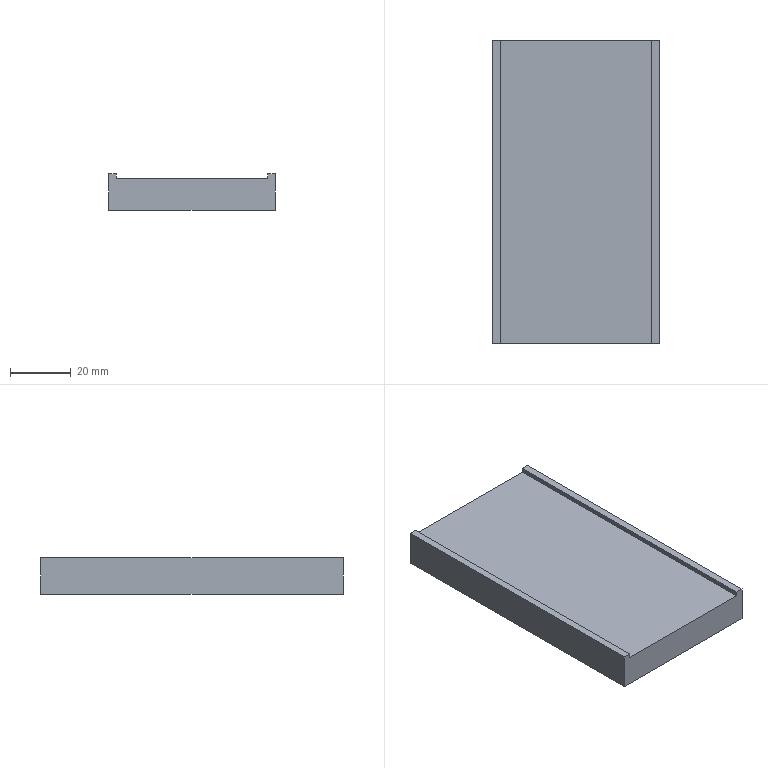Part | SolidWorks | features Extrusion 1, ICE 1 | 1 solid | 10 faces | box 55 x 100 x 12 mm | volume 58500 mm3 | plane 10
STEP:
#1=CARTESIAN_POINT('',(27.5,50.,12.));
#2=VERTEX_POINT('',#1);
#3=CARTESIAN_POINT('',(25.,50.,12.));
#4=VERTEX_POINT('',#3);
#5=CARTESIAN_POINT('',(-27.5,50.,12.));
#6=DIRECTION('',(-1.,0.,0.));
#7=VECTOR('',#6,1000.);
#8=LINE('',#5,#7);
#9=EDGE_CURVE('',#2,#4,#8,.T.);
#10=ORIENTED_EDGE('',*,*,#9,.T.);
#11=CARTESIAN_POINT('',(25.,-50.,12.));
#12=VERTEX_POINT('',#11);
#13=CARTESIAN_POINT('',(25.,-50.,12.));
#14=DIRECTION('',(0.,1.,0.));
#15=VECTOR('',#14,1000.);
#16=LINE('',#13,#15);
#17=EDGE_CURVE('',#12,#4,#16,.T.);
#18=ORIENTED_EDGE('',*,*,#17,.F.);
#19=CARTESIAN_POINT('',(27.5,-50.,12.));
#20=VERTEX_POINT('',#19);
#21=CARTESIAN_POINT('',(-27.5,-50.,12.));
#22=DIRECTION('',(1.,0.,0.));
#23=VECTOR('',#22,1000.);
#24=LINE('',#21,#23);
#25=EDGE_CURVE('',#12,#20,#24,.T.);
#26=ORIENTED_EDGE('',*,*,#25,.T.);
#27=CARTESIAN_POINT('',(27.5,-50.,12.));
#28=DIRECTION('',(0.,1.,0.));
#29=VECTOR('',#28,1000.);
#30=LINE('',#27,#29);
#31=EDGE_CURVE('',#20,#2,#30,.T.);
#32=ORIENTED_EDGE('',*,*,#31,.T.);
#33=EDGE_LOOP('',(#10,#18,#26,#32));
#34=FACE_OUTER_BOUND('',#33,.T.);
#35=CARTESIAN_POINT('',(0.,0.,12.));
#36=DIRECTION('',(0.,0.,-1.));
#37=DIRECTION('',(-1.,0.,0.));
#38=AXIS2_PLACEMENT_3D('',#35,#36,#37);
#39=PLANE('',#38);
#40=ADVANCED_FACE('',(#34),#39,.F.);
#41=CARTESIAN_POINT('',(27.5,-50.,0.));
#42=VERTEX_POINT('',#41);
#43=CARTESIAN_POINT('',(27.5,50.,0.));
#44=VERTEX_POINT('',#43);
#45=CARTESIAN_POINT('',(27.5,-50.,0.));
#46=DIRECTION('',(0.,1.,0.));
#47=VECTOR('',#46,1000.);
#48=LINE('',#45,#47);
#49=EDGE_CURVE('',#42,#44,#48,.T.);
#50=ORIENTED_EDGE('',*,*,#49,.T.);
#51=CARTESIAN_POINT('',(27.5,50.,12.));
#52=DIRECTION('',(0.,0.,-1.));
#53=VECTOR('',#52,1000.);
#54=LINE('',#51,#53);
#55=EDGE_CURVE('',#2,#44,#54,.T.);
#56=ORIENTED_EDGE('',*,*,#55,.F.);
#57=ORIENTED_EDGE('',*,*,#31,.F.);
#58=CARTESIAN_POINT('',(27.5,-50.,12.));
#59=DIRECTION('',(0.,0.,-1.));
#60=VECTOR('',#59,1000.);
#61=LINE('',#58,#60);
#62=EDGE_CURVE('',#20,#42,#61,.T.);
#63=ORIENTED_EDGE('',*,*,#62,.T.);
#64=EDGE_LOOP('',(#50,#56,#57,#63));
#65=FACE_OUTER_BOUND('',#64,.T.);
#66=CARTESIAN_POINT('',(27.5,-50.,12.));
#67=DIRECTION('',(-1.,0.,0.));
#68=DIRECTION('',(0.,0.,1.));
#69=AXIS2_PLACEMENT_3D('',#66,#67,#68);
#70=PLANE('',#69);
#71=ADVANCED_FACE('',(#65),#70,.F.);
#72=CARTESIAN_POINT('',(25.,50.,10.5));
#73=VERTEX_POINT('',#72);
#74=CARTESIAN_POINT('',(-25.,50.,10.5));
#75=VERTEX_POINT('',#74);
#76=CARTESIAN_POINT('',(-25.,50.,10.5));
#77=DIRECTION('',(-1.,0.,0.));
#78=VECTOR('',#77,1000.);
#79=LINE('',#76,#78);
#80=EDGE_CURVE('',#73,#75,#79,.T.);
#81=ORIENTED_EDGE('',*,*,#80,.F.);
#82=CARTESIAN_POINT('',(25.,50.,10.5));
#83=DIRECTION('',(0.,0.,1.));
#84=VECTOR('',#83,1000.);
#85=LINE('',#82,#84);
#86=EDGE_CURVE('',#73,#4,#85,.T.);
#87=ORIENTED_EDGE('',*,*,#86,.T.);
#88=ORIENTED_EDGE('',*,*,#9,.F.);
#89=ORIENTED_EDGE('',*,*,#55,.T.);
#90=CARTESIAN_POINT('',(-27.5,50.,0.));
#91=VERTEX_POINT('',#90);
#92=CARTESIAN_POINT('',(-27.5,50.,0.));
#93=DIRECTION('',(-1.,0.,0.));
#94=VECTOR('',#93,1000.);
#95=LINE('',#92,#94);
#96=EDGE_CURVE('',#44,#91,#95,.T.);
#97=ORIENTED_EDGE('',*,*,#96,.T.);
#98=CARTESIAN_POINT('',(-27.5,50.,12.));
#99=VERTEX_POINT('',#98);
#100=CARTESIAN_POINT('',(-27.5,50.,12.));
#101=DIRECTION('',(0.,0.,-1.));
#102=VECTOR('',#101,1000.);
#103=LINE('',#100,#102);
#104=EDGE_CURVE('',#99,#91,#103,.T.);
#105=ORIENTED_EDGE('',*,*,#104,.F.);
#106=CARTESIAN_POINT('',(-25.,50.,12.));
#107=VERTEX_POINT('',#106);
#108=CARTESIAN_POINT('',(-27.5,50.,12.));
#109=DIRECTION('',(-1.,0.,0.));
#110=VECTOR('',#109,1000.);
#111=LINE('',#108,#110);
#112=EDGE_CURVE('',#107,#99,#111,.T.);
#113=ORIENTED_EDGE('',*,*,#112,.F.);
#114=CARTESIAN_POINT('',(-25.,50.,10.5));
#115=DIRECTION('',(0.,0.,1.));
#116=VECTOR('',#115,1000.);
#117=LINE('',#114,#116);
#118=EDGE_CURVE('',#75,#107,#117,.T.);
#119=ORIENTED_EDGE('',*,*,#118,.F.);
#120=EDGE_LOOP('',(#81,#87,#88,#89,#97,#105,#113,#119));
#121=FACE_OUTER_BOUND('',#120,.T.);
#122=CARTESIAN_POINT('',(-27.5,50.,12.));
#123=DIRECTION('',(0.,-1.,0.));
#124=DIRECTION('',(0.,0.,-1.));
#125=AXIS2_PLACEMENT_3D('',#122,#123,#124);
#126=PLANE('',#125);
#127=ADVANCED_FACE('',(#121),#126,.F.);
#128=CARTESIAN_POINT('',(-27.5,-50.,0.));
#129=VERTEX_POINT('',#128);
#130=CARTESIAN_POINT('',(-27.5,-50.,0.));
#131=DIRECTION('',(0.,-1.,0.));
#132=VECTOR('',#131,1000.);
#133=LINE('',#130,#132);
#134=EDGE_CURVE('',#91,#129,#133,.T.);
#135=ORIENTED_EDGE('',*,*,#134,.T.);
#136=CARTESIAN_POINT('',(-27.5,-50.,12.));
#137=VERTEX_POINT('',#136);
#138=CARTESIAN_POINT('',(-27.5,-50.,12.));
#139=DIRECTION('',(0.,0.,-1.));
#140=VECTOR('',#139,1000.);
#141=LINE('',#138,#140);
#142=EDGE_CURVE('',#137,#129,#141,.T.);
#143=ORIENTED_EDGE('',*,*,#142,.F.);
#144=CARTESIAN_POINT('',(-27.5,-50.,12.));
#145=DIRECTION('',(0.,-1.,0.));
#146=VECTOR('',#145,1000.);
#147=LINE('',#144,#146);
#148=EDGE_CURVE('',#99,#137,#147,.T.);
#149=ORIENTED_EDGE('',*,*,#148,.F.);
#150=ORIENTED_EDGE('',*,*,#104,.T.);
#151=EDGE_LOOP('',(#135,#143,#149,#150));
#152=FACE_OUTER_BOUND('',#151,.T.);
#153=CARTESIAN_POINT('',(-27.5,-50.,12.));
#154=DIRECTION('',(1.,0.,0.));
#155=DIRECTION('',(0.,0.,-1.));
#156=AXIS2_PLACEMENT_3D('',#153,#154,#155);
#157=PLANE('',#156);
#158=ADVANCED_FACE('',(#152),#157,.F.);
#159=ORIENTED_EDGE('',*,*,#25,.F.);
#160=CARTESIAN_POINT('',(25.,-50.,10.5));
#161=VERTEX_POINT('',#160);
#162=CARTESIAN_POINT('',(25.,-50.,10.5));
#163=DIRECTION('',(0.,0.,1.));
#164=VECTOR('',#163,1000.);
#165=LINE('',#162,#164);
#166=EDGE_CURVE('',#161,#12,#165,.T.);
#167=ORIENTED_EDGE('',*,*,#166,.F.);
#168=CARTESIAN_POINT('',(-25.,-50.,10.5));
#169=VERTEX_POINT('',#168);
#170=CARTESIAN_POINT('',(-25.,-50.,10.5));
#171=DIRECTION('',(1.,0.,0.));
#172=VECTOR('',#171,1000.);
#173=LINE('',#170,#172);
#174=EDGE_CURVE('',#169,#161,#173,.T.);
#175=ORIENTED_EDGE('',*,*,#174,.F.);
#176=CARTESIAN_POINT('',(-25.,-50.,12.));
#177=VERTEX_POINT('',#176);
#178=CARTESIAN_POINT('',(-25.,-50.,10.5));
#179=DIRECTION('',(0.,0.,1.));
#180=VECTOR('',#179,1000.);
#181=LINE('',#178,#180);
#182=EDGE_CURVE('',#169,#177,#181,.T.);
#183=ORIENTED_EDGE('',*,*,#182,.T.);
#184=CARTESIAN_POINT('',(-27.5,-50.,12.));
#185=DIRECTION('',(1.,0.,0.));
#186=VECTOR('',#185,1000.);
#187=LINE('',#184,#186);
#188=EDGE_CURVE('',#137,#177,#187,.T.);
#189=ORIENTED_EDGE('',*,*,#188,.F.);
#190=ORIENTED_EDGE('',*,*,#142,.T.);
#191=CARTESIAN_POINT('',(-27.5,-50.,0.));
#192=DIRECTION('',(1.,0.,0.));
#193=VECTOR('',#192,1000.);
#194=LINE('',#191,#193);
#195=EDGE_CURVE('',#129,#42,#194,.T.);
#196=ORIENTED_EDGE('',*,*,#195,.T.);
#197=ORIENTED_EDGE('',*,*,#62,.F.);
#198=EDGE_LOOP('',(#159,#167,#175,#183,#189,#190,#196,#197));
#199=FACE_OUTER_BOUND('',#198,.T.);
#200=CARTESIAN_POINT('',(-27.5,-50.,12.));
#201=DIRECTION('',(0.,1.,0.));
#202=DIRECTION('',(0.,0.,1.));
#203=AXIS2_PLACEMENT_3D('',#200,#201,#202);
#204=PLANE('',#203);
#205=ADVANCED_FACE('',(#199),#204,.F.);
#206=ORIENTED_EDGE('',*,*,#188,.T.);
#207=CARTESIAN_POINT('',(-25.,-50.,12.));
#208=DIRECTION('',(0.,-1.,0.));
#209=VECTOR('',#208,1000.);
#210=LINE('',#207,#209);
#211=EDGE_CURVE('',#107,#177,#210,.T.);
#212=ORIENTED_EDGE('',*,*,#211,.F.);
#213=ORIENTED_EDGE('',*,*,#112,.T.);
#214=ORIENTED_EDGE('',*,*,#148,.T.);
#215=EDGE_LOOP('',(#206,#212,#213,#214));
#216=FACE_OUTER_BOUND('',#215,.T.);
#217=CARTESIAN_POINT('',(0.,0.,12.));
#218=DIRECTION('',(0.,0.,-1.));
#219=DIRECTION('',(-1.,0.,0.));
#220=AXIS2_PLACEMENT_3D('',#217,#218,#219);
#221=PLANE('',#220);
#222=ADVANCED_FACE('',(#216),#221,.F.);
#223=ORIENTED_EDGE('',*,*,#49,.F.);
#224=ORIENTED_EDGE('',*,*,#195,.F.);
#225=ORIENTED_EDGE('',*,*,#134,.F.);
#226=ORIENTED_EDGE('',*,*,#96,.F.);
#227=EDGE_LOOP('',(#223,#224,#225,#226));
#228=FACE_OUTER_BOUND('',#227,.T.);
#229=CARTESIAN_POINT('',(0.,0.,0.));
#230=DIRECTION('',(0.,0.,-1.));
#231=DIRECTION('',(-1.,0.,0.));
#232=AXIS2_PLACEMENT_3D('',#229,#230,#231);
#233=PLANE('',#232);
#234=ADVANCED_FACE('',(#228),#233,.T.);
#235=ORIENTED_EDGE('',*,*,#17,.T.);
#236=ORIENTED_EDGE('',*,*,#86,.F.);
#237=CARTESIAN_POINT('',(25.,-50.,10.5));
#238=DIRECTION('',(0.,1.,0.));
#239=VECTOR('',#238,1000.);
#240=LINE('',#237,#239);
#241=EDGE_CURVE('',#161,#73,#240,.T.);
#242=ORIENTED_EDGE('',*,*,#241,.F.);
#243=ORIENTED_EDGE('',*,*,#166,.T.);
#244=EDGE_LOOP('',(#235,#236,#242,#243));
#245=FACE_OUTER_BOUND('',#244,.T.);
#246=CARTESIAN_POINT('',(25.,-50.,10.5));
#247=DIRECTION('',(1.,0.,0.));
#248=DIRECTION('',(0.,0.,-1.));
#249=AXIS2_PLACEMENT_3D('',#246,#247,#248);
#250=PLANE('',#249);
#251=ADVANCED_FACE('',(#245),#250,.F.);
#252=ORIENTED_EDGE('',*,*,#211,.T.);
#253=ORIENTED_EDGE('',*,*,#182,.F.);
#254=CARTESIAN_POINT('',(-25.,-50.,10.5));
#255=DIRECTION('',(0.,-1.,0.));
#256=VECTOR('',#255,1000.);
#257=LINE('',#254,#256);
#258=EDGE_CURVE('',#75,#169,#257,.T.);
#259=ORIENTED_EDGE('',*,*,#258,.F.);
#260=ORIENTED_EDGE('',*,*,#118,.T.);
#261=EDGE_LOOP('',(#252,#253,#259,#260));
#262=FACE_OUTER_BOUND('',#261,.T.);
#263=CARTESIAN_POINT('',(-25.,-50.,10.5));
#264=DIRECTION('',(-1.,0.,0.));
#265=DIRECTION('',(0.,0.,1.));
#266=AXIS2_PLACEMENT_3D('',#263,#264,#265);
#267=PLANE('',#266);
#268=ADVANCED_FACE('',(#262),#267,.F.);
#269=ORIENTED_EDGE('',*,*,#241,.T.);
#270=ORIENTED_EDGE('',*,*,#80,.T.);
#271=ORIENTED_EDGE('',*,*,#258,.T.);
#272=ORIENTED_EDGE('',*,*,#174,.T.);
#273=EDGE_LOOP('',(#269,#270,#271,#272));
#274=FACE_OUTER_BOUND('',#273,.T.);
#275=CARTESIAN_POINT('',(0.,0.,10.5));
#276=DIRECTION('',(0.,0.,-1.));
#277=DIRECTION('',(-1.,0.,0.));
#278=AXIS2_PLACEMENT_3D('',#275,#276,#277);
#279=PLANE('',#278);
#280=ADVANCED_FACE('',(#274),#279,.F.);
#281=CLOSED_SHELL('',(#40,#71,#127,#158,#205,#222,#234,#251,#268,#280));
#282=MANIFOLD_SOLID_BREP('',#281);
#283=CARTESIAN_POINT('',(0.,0.,0.));
#284=DIRECTION('',(0.,0.,1.));
#285=DIRECTION('',(1.,0.,0.));
#286=AXIS2_PLACEMENT_3D('',#283,#284,#285);
#287=(LENGTH_UNIT()NAMED_UNIT(*)SI_UNIT(.MILLI.,.METRE.));
#288=UNCERTAINTY_MEASURE_WITH_UNIT(LENGTH_MEASURE(0.00001),#287,'','');
#289=(NAMED_UNIT(*)PLANE_ANGLE_UNIT()SI_UNIT($,.RADIAN.));
#290=(NAMED_UNIT(*)SI_UNIT($,.STERADIAN.)SOLID_ANGLE_UNIT());
#291=(GEOMETRIC_REPRESENTATION_CONTEXT(3)GLOBAL_UNCERTAINTY_ASSIGNED_CONTEXT((#288))GLOBAL_UNIT_ASSIGNED_CONTEXT((#287,#289,#290))REPRESENTATION_CONTEXT('',''));
#292=ADVANCED_BREP_SHAPE_REPRESENTATION('',(#282,#286),#291);